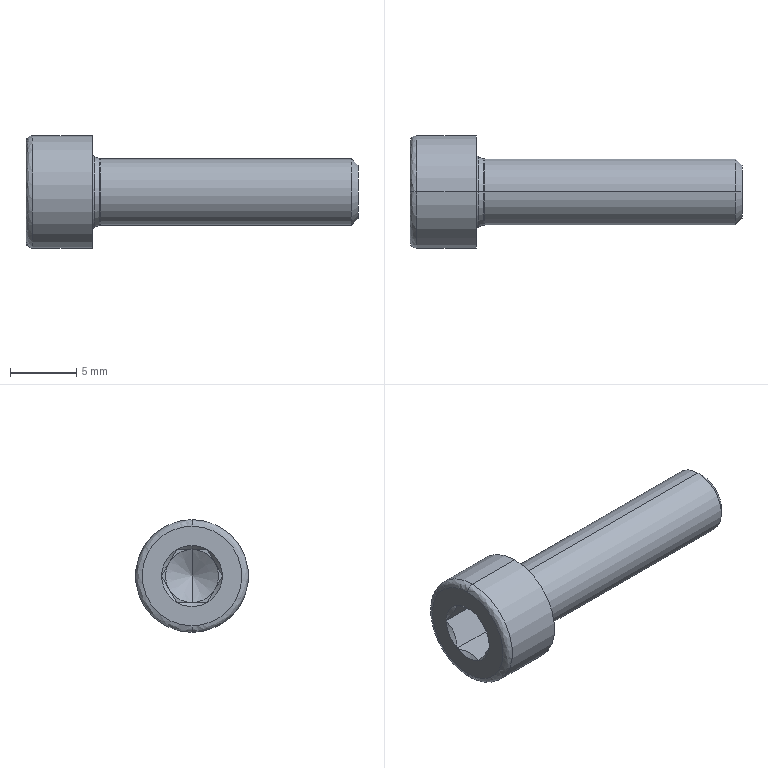Part | STEP file | _Hexagon socket head cap screw DIN 912 - M5x20 | 1 solid | 38 faces | box 25 x 8.5 x 8.5 mm | volume 626.207 mm3 | plane 15 | cone 13 | spline 6 | cylinder 4 | commonest cylinder face diameters 5 x2 8.5 x2
STEP:
#1=CARTESIAN_POINT('',(0.5298,0.,2.513));
#2=VERTEX_POINT('',#1);
#3=CARTESIAN_POINT('',(0.5298,0.,-2.513));
#4=VERTEX_POINT('',#3);
#5=CARTESIAN_POINT('',(0.5298,0.,0.));
#6=DIRECTION('',(-1.,0.,0.));
#7=DIRECTION('',(0.,0.,-1.));
#8=AXIS2_PLACEMENT_3D('',#5,#6,#7);
#9=CIRCLE('',#8,2.513);
#10=EDGE_CURVE('',#2,#4,#9,.T.);
#11=ORIENTED_EDGE('',*,*,#10,.F.);
#12=CARTESIAN_POINT('',(0.6,0.,2.5));
#13=VERTEX_POINT('',#12);
#14=CARTESIAN_POINT('',(0.6,0.,2.7));
#15=DIRECTION('',(0.,-1.,0.));
#16=DIRECTION('',(0.,0.,1.));
#17=AXIS2_PLACEMENT_3D('',#14,#15,#16);
#18=CIRCLE('',#17,0.2);
#19=EDGE_CURVE('',#2,#13,#18,.T.);
#20=ORIENTED_EDGE('',*,*,#19,.T.);
#21=CARTESIAN_POINT('',(0.6,0.,-2.5));
#22=VERTEX_POINT('',#21);
#23=CARTESIAN_POINT('',(0.6,0.,0.));
#24=DIRECTION('',(1.,0.,0.));
#25=DIRECTION('',(0.,0.,1.));
#26=AXIS2_PLACEMENT_3D('',#23,#24,#25);
#27=CIRCLE('',#26,2.5);
#28=EDGE_CURVE('',#22,#13,#27,.T.);
#29=ORIENTED_EDGE('',*,*,#28,.F.);
#30=CARTESIAN_POINT('',(0.6,0.,-2.7));
#31=DIRECTION('',(0.,1.,0.));
#32=DIRECTION('',(0.,0.,-1.));
#33=AXIS2_PLACEMENT_3D('',#30,#31,#32);
#34=CIRCLE('',#33,0.2);
#35=EDGE_CURVE('',#4,#22,#34,.T.);
#36=ORIENTED_EDGE('',*,*,#35,.F.);
#37=EDGE_LOOP('',(#11,#20,#29,#36));
#38=FACE_OUTER_BOUND('',#37,.T.);
#39=CARTESIAN_POINT('',(0.5298,0.,-2.513));
#40=CARTESIAN_POINT('',(0.5298,5.025,-2.513));
#41=CARTESIAN_POINT('',(0.5298,5.025,2.513));
#42=CARTESIAN_POINT('',(0.5298,0.,2.513));
#43=CARTESIAN_POINT('',(0.5523,0.,-2.504));
#44=CARTESIAN_POINT('',(0.5523,5.009,-2.504));
#45=CARTESIAN_POINT('',(0.5523,5.009,2.504));
#46=CARTESIAN_POINT('',(0.5523,0.,2.504));
#47=CARTESIAN_POINT('',(0.576,0.,-2.5));
#48=CARTESIAN_POINT('',(0.576,5.,-2.5));
#49=CARTESIAN_POINT('',(0.576,5.,2.5));
#50=CARTESIAN_POINT('',(0.576,0.,2.5));
#51=CARTESIAN_POINT('',(0.6,0.,-2.5));
#52=CARTESIAN_POINT('',(0.6,5.,-2.5));
#53=CARTESIAN_POINT('',(0.6,5.,2.5));
#54=CARTESIAN_POINT('',(0.6,0.,2.5));
#55=(BOUNDED_SURFACE()B_SPLINE_SURFACE(3,3,((#39,#40,#41,#42),(#43,#44,#45,#46),(#47,#48,#49,#50),(#51,#52,#53,#54)),.UNSPECIFIED.,.F.,.F.,.F.)B_SPLINE_SURFACE_WITH_KNOTS((4,4),(4,4),(0.,1.),(0.,1.),.UNSPECIFIED.)GEOMETRIC_REPRESENTATION_ITEM()RATIONAL_B_SPLINE_SURFACE(((1.,0.3333,0.3333,1.),(0.9893,0.3298,0.3298,0.9893),(0.9893,0.3298,0.3298,0.9893),(1.,0.3333,0.3333,1.)))REPRESENTATION_ITEM('')SURFACE());
#56=ADVANCED_FACE('',(#38),#55,.F.);
#57=CARTESIAN_POINT('',(0.,0.,2.85));
#58=VERTEX_POINT('',#57);
#59=CARTESIAN_POINT('',(0.,0.,-2.85));
#60=VERTEX_POINT('',#59);
#61=CARTESIAN_POINT('',(0.,0.,2.85));
#62=CARTESIAN_POINT('',(0.,0.1814,2.85));
#63=CARTESIAN_POINT('',(0.,0.4486,2.825));
#64=CARTESIAN_POINT('',(0.,0.7517,2.752));
#65=CARTESIAN_POINT('',(0.,0.9011,2.705));
#66=CARTESIAN_POINT('',(0.,0.9647,2.682));
#67=CARTESIAN_POINT('',(0.,1.007,2.666));
#68=CARTESIAN_POINT('',(0.,1.026,2.659));
#69=CARTESIAN_POINT('',(0.,1.415,2.505));
#70=CARTESIAN_POINT('',(0.,1.737,2.294));
#71=CARTESIAN_POINT('',(0.,2.154,1.876));
#72=CARTESIAN_POINT('',(0.,2.338,1.651));
#73=CARTESIAN_POINT('',(0.,2.509,1.359));
#74=CARTESIAN_POINT('',(0.,2.583,1.207));
#75=CARTESIAN_POINT('',(0.,2.612,1.14));
#76=CARTESIAN_POINT('',(0.,2.632,1.095));
#77=CARTESIAN_POINT('',(0.,2.642,1.07));
#78=CARTESIAN_POINT('',(0.,2.783,0.7118));
#79=CARTESIAN_POINT('',(0.,2.85,0.3628));
#80=CARTESIAN_POINT('',(0.,2.85,-0.1814));
#81=CARTESIAN_POINT('',(0.,2.825,-0.4486));
#82=CARTESIAN_POINT('',(0.,2.752,-0.7517));
#83=CARTESIAN_POINT('',(0.,2.705,-0.9011));
#84=CARTESIAN_POINT('',(0.,2.682,-0.9647));
#85=CARTESIAN_POINT('',(0.,2.666,-1.007));
#86=CARTESIAN_POINT('',(0.,2.659,-1.026));
#87=CARTESIAN_POINT('',(0.,2.505,-1.415));
#88=CARTESIAN_POINT('',(0.,2.294,-1.737));
#89=CARTESIAN_POINT('',(0.,1.876,-2.154));
#90=CARTESIAN_POINT('',(0.,1.651,-2.338));
#91=CARTESIAN_POINT('',(0.,1.359,-2.509));
#92=CARTESIAN_POINT('',(0.,1.207,-2.583));
#93=CARTESIAN_POINT('',(0.,1.14,-2.612));
#94=CARTESIAN_POINT('',(0.,1.095,-2.632));
#95=CARTESIAN_POINT('',(0.,1.07,-2.642));
#96=CARTESIAN_POINT('',(0.,0.7119,-2.783));
#97=CARTESIAN_POINT('',(0.,0.3622,-2.85));
#98=CARTESIAN_POINT('',(0.,0.,-2.85));
#99=B_SPLINE_CURVE_WITH_KNOTS('',3,(#61,#62,#63,#64,#65,#66,#67,#68,#69,#70,#71,#72,#73,#74,#75,#76,#77,#78,#79,#80,#81,#82,#83,#84,#85,#86,#87,#88,#89,#90,#91,#92,#93,#94,#95,#96,#97,#98),.UNSPECIFIED.,.F.,.F.,(4,1,1,1,2,2,2,1,1,1,2,2,2,1,1,1,2,2,2,1,1,1,2,2,4),(0.5,0.5312,0.5469,0.5547,0.5586,0.5625,0.625,0.6562,0.6719,0.6797,0.6836,0.6875,0.75,0.7812,0.7969,0.8047,0.8086,0.8125,0.875,0.9062,0.9219,0.9297,0.9336,0.9375,1.),.UNSPECIFIED.);
#100=EDGE_CURVE('',#58,#60,#99,.T.);
#101=ORIENTED_EDGE('',*,*,#100,.F.);
#102=CARTESIAN_POINT('',(0.1298,0.,2.663));
#103=VERTEX_POINT('',#102);
#104=CARTESIAN_POINT('',(0.2,0.,2.85));
#105=DIRECTION('',(0.,-1.,0.));
#106=DIRECTION('',(0.,0.,1.));
#107=AXIS2_PLACEMENT_3D('',#104,#105,#106);
#108=CIRCLE('',#107,0.2);
#109=EDGE_CURVE('',#58,#103,#108,.T.);
#110=ORIENTED_EDGE('',*,*,#109,.T.);
#111=CARTESIAN_POINT('',(0.1298,0.,-2.663));
#112=VERTEX_POINT('',#111);
#113=CARTESIAN_POINT('',(0.1298,0.,0.));
#114=DIRECTION('',(1.,0.,0.));
#115=DIRECTION('',(0.,0.,1.));
#116=AXIS2_PLACEMENT_3D('',#113,#114,#115);
#117=CIRCLE('',#116,2.663);
#118=EDGE_CURVE('',#112,#103,#117,.T.);
#119=ORIENTED_EDGE('',*,*,#118,.F.);
#120=CARTESIAN_POINT('',(0.2,0.,-2.85));
#121=DIRECTION('',(0.,1.,0.));
#122=DIRECTION('',(0.,0.,-1.));
#123=AXIS2_PLACEMENT_3D('',#120,#121,#122);
#124=CIRCLE('',#123,0.2);
#125=EDGE_CURVE('',#60,#112,#124,.T.);
#126=ORIENTED_EDGE('',*,*,#125,.F.);
#127=EDGE_LOOP('',(#101,#110,#119,#126));
#128=FACE_OUTER_BOUND('',#127,.T.);
#129=CARTESIAN_POINT('',(0.,0.,-2.85));
#130=CARTESIAN_POINT('',(0.,5.7,-2.85));
#131=CARTESIAN_POINT('',(0.,5.7,2.85));
#132=CARTESIAN_POINT('',(0.,0.,2.85));
#133=CARTESIAN_POINT('',(0.,0.,-2.764));
#134=CARTESIAN_POINT('',(0.,5.528,-2.764));
#135=CARTESIAN_POINT('',(0.,5.528,2.764));
#136=CARTESIAN_POINT('',(0.,0.,2.764));
#137=CARTESIAN_POINT('',(0.04909,0.,-2.693));
#138=CARTESIAN_POINT('',(0.04909,5.386,-2.693));
#139=CARTESIAN_POINT('',(0.04909,5.386,2.693));
#140=CARTESIAN_POINT('',(0.04909,0.,2.693));
#141=CARTESIAN_POINT('',(0.1298,0.,-2.663));
#142=CARTESIAN_POINT('',(0.1298,5.325,-2.663));
#143=CARTESIAN_POINT('',(0.1298,5.325,2.663));
#144=CARTESIAN_POINT('',(0.1298,0.,2.663));
#145=(BOUNDED_SURFACE()B_SPLINE_SURFACE(3,3,((#129,#130,#131,#132),(#133,#134,#135,#136),(#137,#138,#139,#140),(#141,#142,#143,#144)),.UNSPECIFIED.,.F.,.F.,.F.)B_SPLINE_SURFACE_WITH_KNOTS((4,4),(4,4),(0.,1.),(0.,1.),.UNSPECIFIED.)GEOMETRIC_REPRESENTATION_ITEM()RATIONAL_B_SPLINE_SURFACE(((1.,0.3333,0.3333,1.),(0.8813,0.2938,0.2938,0.8813),(0.8813,0.2938,0.2938,0.8813),(1.,0.3333,0.3333,1.)))REPRESENTATION_ITEM('')SURFACE());
#146=ADVANCED_FACE('',(#128),#145,.F.);
#147=CARTESIAN_POINT('',(-4.5,0.,4.25));
#148=VERTEX_POINT('',#147);
#149=CARTESIAN_POINT('',(-4.5,0.,-4.25));
#150=VERTEX_POINT('',#149);
#151=CARTESIAN_POINT('',(-4.5,0.,0.));
#152=DIRECTION('',(1.,0.,0.));
#153=DIRECTION('',(0.,0.,1.));
#154=AXIS2_PLACEMENT_3D('',#151,#152,#153);
#155=CIRCLE('',#154,4.25);
#156=EDGE_CURVE('',#148,#150,#155,.T.);
#157=ORIENTED_EDGE('',*,*,#156,.F.);
#158=CARTESIAN_POINT('',(-5.,0.,3.75));
#159=VERTEX_POINT('',#158);
#160=CARTESIAN_POINT('',(-4.5,0.,3.75));
#161=DIRECTION('',(0.,-1.,0.));
#162=DIRECTION('',(0.,0.,1.));
#163=AXIS2_PLACEMENT_3D('',#160,#161,#162);
#164=CIRCLE('',#163,0.5);
#165=EDGE_CURVE('',#148,#159,#164,.T.);
#166=ORIENTED_EDGE('',*,*,#165,.T.);
#167=CARTESIAN_POINT('',(-5.,0.,-3.75));
#168=VERTEX_POINT('',#167);
#169=CARTESIAN_POINT('',(-5.,0.,3.75));
#170=CARTESIAN_POINT('',(-5.,-7.5,3.75));
#171=CARTESIAN_POINT('',(-5.,-7.5,-3.75));
#172=CARTESIAN_POINT('',(-5.,0.,-3.75));
#173=(BOUNDED_CURVE()B_SPLINE_CURVE(3,(#169,#170,#171,#172),.UNSPECIFIED.,.F.,.T.)B_SPLINE_CURVE_WITH_KNOTS((4,4),(0.5,1.),.UNSPECIFIED.)CURVE()GEOMETRIC_REPRESENTATION_ITEM()RATIONAL_B_SPLINE_CURVE((1.,0.3333,0.3333,1.))REPRESENTATION_ITEM(''));
#174=EDGE_CURVE('',#159,#168,#173,.T.);
#175=ORIENTED_EDGE('',*,*,#174,.T.);
#176=CARTESIAN_POINT('',(-4.5,0.,-3.75));
#177=DIRECTION('',(0.,1.,0.));
#178=DIRECTION('',(0.,0.,-1.));
#179=AXIS2_PLACEMENT_3D('',#176,#177,#178);
#180=CIRCLE('',#179,0.5);
#181=EDGE_CURVE('',#150,#168,#180,.T.);
#182=ORIENTED_EDGE('',*,*,#181,.F.);
#183=EDGE_LOOP('',(#157,#166,#175,#182));
#184=FACE_OUTER_BOUND('',#183,.T.);
#185=CARTESIAN_POINT('',(-4.5,0.,4.25));
#186=CARTESIAN_POINT('',(-4.5,-8.5,4.25));
#187=CARTESIAN_POINT('',(-4.5,-8.5,-4.25));
#188=CARTESIAN_POINT('',(-4.5,0.,-4.25));
#189=CARTESIAN_POINT('',(-4.793,0.,4.25));
#190=CARTESIAN_POINT('',(-4.793,-8.5,4.25));
#191=CARTESIAN_POINT('',(-4.793,-8.5,-4.25));
#192=CARTESIAN_POINT('',(-4.793,0.,-4.25));
#193=CARTESIAN_POINT('',(-5.,0.,4.043));
#194=CARTESIAN_POINT('',(-5.,-8.086,4.043));
#195=CARTESIAN_POINT('',(-5.,-8.086,-4.043));
#196=CARTESIAN_POINT('',(-5.,0.,-4.043));
#197=CARTESIAN_POINT('',(-5.,0.,3.75));
#198=CARTESIAN_POINT('',(-5.,-7.5,3.75));
#199=CARTESIAN_POINT('',(-5.,-7.5,-3.75));
#200=CARTESIAN_POINT('',(-5.,0.,-3.75));
#201=(BOUNDED_SURFACE()B_SPLINE_SURFACE(3,3,((#185,#186,#187,#188),(#189,#190,#191,#192),(#193,#194,#195,#196),(#197,#198,#199,#200)),.UNSPECIFIED.,.F.,.F.,.F.)B_SPLINE_SURFACE_WITH_KNOTS((4,4),(4,4),(0.,1.),(0.,1.),.UNSPECIFIED.)GEOMETRIC_REPRESENTATION_ITEM()RATIONAL_B_SPLINE_SURFACE(((1.,0.3333,0.3333,1.),(0.8047,0.2682,0.2682,0.8047),(0.8047,0.2682,0.2682,0.8047),(1.,0.3333,0.3333,1.)))REPRESENTATION_ITEM('')SURFACE());
#202=ADVANCED_FACE('',(#184),#201,.T.);
#203=CARTESIAN_POINT('',(19.509,0.,2.5));
#204=VERTEX_POINT('',#203);
#205=CARTESIAN_POINT('',(19.509,0.,-2.5));
#206=VERTEX_POINT('',#205);
#207=CARTESIAN_POINT('',(19.509,0.,0.));
#208=DIRECTION('',(-1.,0.,0.));
#209=DIRECTION('',(0.,0.,1.));
#210=AXIS2_PLACEMENT_3D('',#207,#208,#209);
#211=CIRCLE('',#210,2.5);
#212=EDGE_CURVE('',#204,#206,#211,.T.);
#213=ORIENTED_EDGE('',*,*,#212,.T.);
#214=CARTESIAN_POINT('',(23.,0.,-2.5));
#215=DIRECTION('',(-1.,0.,0.));
#216=VECTOR('',#215,1000.);
#217=LINE('',#214,#216);
#218=EDGE_CURVE('',#206,#22,#217,.T.);
#219=ORIENTED_EDGE('',*,*,#218,.T.);
#220=ORIENTED_EDGE('',*,*,#28,.T.);
#221=CARTESIAN_POINT('',(23.,0.,2.5));
#222=DIRECTION('',(-1.,0.,0.));
#223=VECTOR('',#222,1000.);
#224=LINE('',#221,#223);
#225=EDGE_CURVE('',#204,#13,#224,.T.);
#226=ORIENTED_EDGE('',*,*,#225,.F.);
#227=EDGE_LOOP('',(#213,#219,#220,#226));
#228=FACE_OUTER_BOUND('',#227,.T.);
#229=CARTESIAN_POINT('',(23.,0.,0.));
#230=DIRECTION('',(-1.,0.,0.));
#231=DIRECTION('',(0.,0.,1.));
#232=AXIS2_PLACEMENT_3D('',#229,#230,#231);
#233=CYLINDRICAL_SURFACE('',#232,2.5);
#234=ADVANCED_FACE('',(#228),#233,.T.);
#235=CARTESIAN_POINT('',(20.,0.,2.009));
#236=VERTEX_POINT('',#235);
#237=CARTESIAN_POINT('',(20.,0.,-2.009));
#238=VERTEX_POINT('',#237);
#239=CARTESIAN_POINT('',(20.,0.,0.));
#240=DIRECTION('',(-1.,0.,0.));
#241=DIRECTION('',(0.,0.,1.));
#242=AXIS2_PLACEMENT_3D('',#239,#240,#241);
#243=CIRCLE('',#242,2.009);
#244=EDGE_CURVE('',#236,#238,#243,.T.);
#245=ORIENTED_EDGE('',*,*,#244,.T.);
#246=CARTESIAN_POINT('',(19.509,0.,-2.5));
#247=DIRECTION('',(-0.7071,0.,-0.7071));
#248=VECTOR('',#247,1000.);
#249=LINE('',#246,#248);
#250=EDGE_CURVE('',#238,#206,#249,.T.);
#251=ORIENTED_EDGE('',*,*,#250,.T.);
#252=ORIENTED_EDGE('',*,*,#212,.F.);
#253=CARTESIAN_POINT('',(19.509,0.,2.5));
#254=DIRECTION('',(-0.7071,0.,0.7071));
#255=VECTOR('',#254,1000.);
#256=LINE('',#253,#255);
#257=EDGE_CURVE('',#236,#204,#256,.T.);
#258=ORIENTED_EDGE('',*,*,#257,.F.);
#259=EDGE_LOOP('',(#245,#251,#252,#258));
#260=FACE_OUTER_BOUND('',#259,.T.);
#261=CARTESIAN_POINT('',(19.509,0.,0.));
#262=DIRECTION('',(-1.,0.,0.));
#263=DIRECTION('',(0.,0.,1.));
#264=AXIS2_PLACEMENT_3D('',#261,#262,#263);
#265=CONICAL_SURFACE('',#264,2.5,0.7854);
#266=ADVANCED_FACE('',(#260),#265,.T.);
#267=ORIENTED_EDGE('',*,*,#10,.T.);
#268=CARTESIAN_POINT('',(0.1298,0.,-2.663));
#269=DIRECTION('',(-0.9363,0.,-0.3511));
#270=VECTOR('',#269,1000.);
#271=LINE('',#268,#270);
#272=EDGE_CURVE('',#4,#112,#271,.T.);
#273=ORIENTED_EDGE('',*,*,#272,.T.);
#274=ORIENTED_EDGE('',*,*,#118,.T.);
#275=CARTESIAN_POINT('',(0.1298,0.,2.663));
#276=DIRECTION('',(-0.9363,0.,0.3511));
#277=VECTOR('',#276,1000.);
#278=LINE('',#275,#277);
#279=EDGE_CURVE('',#2,#103,#278,.T.);
#280=ORIENTED_EDGE('',*,*,#279,.F.);
#281=EDGE_LOOP('',(#267,#273,#274,#280));
#282=FACE_OUTER_BOUND('',#281,.T.);
#283=CARTESIAN_POINT('',(0.1298,0.,0.));
#284=DIRECTION('',(-1.,0.,0.));
#285=DIRECTION('',(0.,0.,1.));
#286=AXIS2_PLACEMENT_3D('',#283,#284,#285);
#287=CONICAL_SURFACE('',#286,2.663,0.3588);
#288=ADVANCED_FACE('',(#282),#287,.T.);
#289=CARTESIAN_POINT('',(0.,0.,4.25));
#290=VERTEX_POINT('',#289);
#291=CARTESIAN_POINT('',(0.,0.,-4.25));
#292=VERTEX_POINT('',#291);
#293=CARTESIAN_POINT('',(0.,0.,0.));
#294=DIRECTION('',(-1.,0.,0.));
#295=DIRECTION('',(0.,0.,1.));
#296=AXIS2_PLACEMENT_3D('',#293,#294,#295);
#297=CIRCLE('',#296,4.25);
#298=EDGE_CURVE('',#290,#292,#297,.T.);
#299=ORIENTED_EDGE('',*,*,#298,.T.);
#300=CARTESIAN_POINT('',(23.,0.,-4.25));
#301=DIRECTION('',(-1.,0.,0.));
#302=VECTOR('',#301,1000.);
#303=LINE('',#300,#302);
#304=EDGE_CURVE('',#292,#150,#303,.T.);
#305=ORIENTED_EDGE('',*,*,#304,.T.);
#306=CARTESIAN_POINT('',(-4.5,0.,0.));
#307=DIRECTION('',(1.,0.,0.));
#308=DIRECTION('',(0.,0.,1.));
#309=AXIS2_PLACEMENT_3D('',#306,#307,#308);
#310=CIRCLE('',#309,4.25);
#311=EDGE_CURVE('',#150,#148,#310,.T.);
#312=ORIENTED_EDGE('',*,*,#311,.T.);
#313=CARTESIAN_POINT('',(23.,0.,4.25));
#314=DIRECTION('',(-1.,0.,0.));
#315=VECTOR('',#314,1000.);
#316=LINE('',#313,#315);
#317=EDGE_CURVE('',#290,#148,#316,.T.);
#318=ORIENTED_EDGE('',*,*,#317,.F.);
#319=EDGE_LOOP('',(#299,#305,#312,#318));
#320=FACE_OUTER_BOUND('',#319,.T.);
#321=CARTESIAN_POINT('',(23.,0.,0.));
#322=DIRECTION('',(-1.,0.,0.));
#323=DIRECTION('',(0.,0.,1.));
#324=AXIS2_PLACEMENT_3D('',#321,#322,#323);
#325=CYLINDRICAL_SURFACE('',#324,4.25);
#326=ADVANCED_FACE('',(#320),#325,.T.);
#327=CARTESIAN_POINT('',(-4.71,0.,2.));
#328=VERTEX_POINT('',#327);
#329=CARTESIAN_POINT('',(-5.,1.115,2.));
#330=VERTEX_POINT('',#329);
#331=CARTESIAN_POINT('',(-4.71,0.,2.));
#332=CARTESIAN_POINT('',(-4.71,0.3872,2.));
#333=CARTESIAN_POINT('',(-4.829,0.765,2.));
#334=CARTESIAN_POINT('',(-5.,1.115,2.));
#335=B_SPLINE_CURVE_WITH_KNOTS('',3,(#331,#332,#333,#334),.UNSPECIFIED.,.F.,.F.,(4,4),(0.001154,0.0023),.UNSPECIFIED.);
#336=EDGE_CURVE('',#328,#330,#335,.T.);
#337=ORIENTED_EDGE('',*,*,#336,.F.);
#338=CARTESIAN_POINT('',(-5.,0.,2.29));
#339=VERTEX_POINT('',#338);
#340=CARTESIAN_POINT('',(-5.,0.,2.29));
#341=DIRECTION('',(-0.7071,0.,0.7071));
#342=VECTOR('',#341,1000.);
#343=LINE('',#340,#342);
#344=EDGE_CURVE('',#328,#339,#343,.T.);
#345=ORIENTED_EDGE('',*,*,#344,.T.);
#346=CARTESIAN_POINT('',(-5.,0.,0.));
#347=DIRECTION('',(-1.,0.,0.));
#348=DIRECTION('',(0.,0.,1.));
#349=AXIS2_PLACEMENT_3D('',#346,#347,#348);
#350=CIRCLE('',#349,2.29);
#351=EDGE_CURVE('',#339,#330,#350,.T.);
#352=ORIENTED_EDGE('',*,*,#351,.T.);
#353=EDGE_LOOP('',(#337,#345,#352));
#354=FACE_OUTER_BOUND('',#353,.T.);
#355=CARTESIAN_POINT('',(-5.,0.,0.));
#356=DIRECTION('',(-1.,0.,0.));
#357=DIRECTION('',(0.,0.,1.));
#358=AXIS2_PLACEMENT_3D('',#355,#356,#357);
#359=CONICAL_SURFACE('',#358,2.29,0.7854);
#360=ADVANCED_FACE('',(#354),#359,.F.);
#361=CARTESIAN_POINT('',(-0.7453,0.,0.));
#362=VERTEX_POINT('',#361);
#363=CARTESIAN_POINT('',(-1.9,0.,2.));
#364=VERTEX_POINT('',#363);
#365=CARTESIAN_POINT('',(-1.9,0.,2.));
#366=DIRECTION('',(-0.5,0.,0.866));
#367=VECTOR('',#366,1000.);
#368=LINE('',#365,#367);
#369=EDGE_CURVE('',#362,#364,#368,.T.);
#370=ORIENTED_EDGE('',*,*,#369,.F.);
#371=CARTESIAN_POINT('',(-1.9,0.,-2.));
#372=VERTEX_POINT('',#371);
#373=CARTESIAN_POINT('',(-1.9,0.,-2.));
#374=DIRECTION('',(-0.5,0.,-0.866));
#375=VECTOR('',#374,1000.);
#376=LINE('',#373,#375);
#377=EDGE_CURVE('',#362,#372,#376,.T.);
#378=ORIENTED_EDGE('',*,*,#377,.T.);
#379=CARTESIAN_POINT('',(-1.9,-1.732,-1.));
#380=VERTEX_POINT('',#379);
#381=CARTESIAN_POINT('',(-1.9,0.,0.));
#382=DIRECTION('',(1.,0.,0.));
#383=DIRECTION('',(0.,0.,1.));
#384=AXIS2_PLACEMENT_3D('',#381,#382,#383);
#385=CIRCLE('',#384,2.);
#386=EDGE_CURVE('',#380,#372,#385,.T.);
#387=ORIENTED_EDGE('',*,*,#386,.F.);
#388=CARTESIAN_POINT('',(-1.9,-1.732,1.));
#389=VERTEX_POINT('',#388);
#390=CARTESIAN_POINT('',(-1.9,0.,0.));
#391=DIRECTION('',(1.,0.,0.));
#392=DIRECTION('',(0.,0.,1.));
#393=AXIS2_PLACEMENT_3D('',#390,#391,#392);
#394=CIRCLE('',#393,2.);
#395=EDGE_CURVE('',#389,#380,#394,.T.);
#396=ORIENTED_EDGE('',*,*,#395,.F.);
#397=CARTESIAN_POINT('',(-1.9,0.,0.));
#398=DIRECTION('',(1.,0.,0.));
#399=DIRECTION('',(0.,0.,1.));
#400=AXIS2_PLACEMENT_3D('',#397,#398,#399);
#401=CIRCLE('',#400,2.);
#402=EDGE_CURVE('',#364,#389,#401,.T.);
#403=ORIENTED_EDGE('',*,*,#402,.F.);
#404=EDGE_LOOP('',(#370,#378,#387,#396,#403));
#405=FACE_OUTER_BOUND('',#404,.T.);
#406=CARTESIAN_POINT('',(-1.9,0.,0.));
#407=DIRECTION('',(-1.,0.,0.));
#408=DIRECTION('',(0.,0.,1.));
#409=AXIS2_PLACEMENT_3D('',#406,#407,#408);
#410=CONICAL_SURFACE('',#409,2.,1.047);
#411=ADVANCED_FACE('',(#405),#410,.F.);
#412=ORIENTED_EDGE('',*,*,#218,.F.);
#413=CARTESIAN_POINT('',(19.509,0.,0.));
#414=DIRECTION('',(-1.,0.,0.));
#415=DIRECTION('',(0.,0.,1.));
#416=AXIS2_PLACEMENT_3D('',#413,#414,#415);
#417=CIRCLE('',#416,2.5);
#418=EDGE_CURVE('',#206,#204,#417,.T.);
#419=ORIENTED_EDGE('',*,*,#418,.T.);
#420=ORIENTED_EDGE('',*,*,#225,.T.);
#421=CARTESIAN_POINT('',(0.6,0.,0.));
#422=DIRECTION('',(1.,0.,0.));
#423=DIRECTION('',(0.,0.,1.));
#424=AXIS2_PLACEMENT_3D('',#421,#422,#423);
#425=CIRCLE('',#424,2.5);
#426=EDGE_CURVE('',#13,#22,#425,.T.);
#427=ORIENTED_EDGE('',*,*,#426,.T.);
#428=EDGE_LOOP('',(#412,#419,#420,#427));
#429=FACE_OUTER_BOUND('',#428,.T.);
#430=CARTESIAN_POINT('',(23.,0.,0.));
#431=DIRECTION('',(-1.,0.,0.));
#432=DIRECTION('',(0.,0.,1.));
#433=AXIS2_PLACEMENT_3D('',#430,#431,#432);
#434=CYLINDRICAL_SURFACE('',#433,2.5);
#435=ADVANCED_FACE('',(#429),#434,.T.);
#436=ORIENTED_EDGE('',*,*,#19,.F.);
#437=CARTESIAN_POINT('',(0.5298,0.,0.));
#438=DIRECTION('',(-1.,0.,0.));
#439=DIRECTION('',(0.,0.,-1.));
#440=AXIS2_PLACEMENT_3D('',#437,#438,#439);
#441=CIRCLE('',#440,2.513);
#442=EDGE_CURVE('',#4,#2,#441,.T.);
#443=ORIENTED_EDGE('',*,*,#442,.F.);
#444=ORIENTED_EDGE('',*,*,#35,.T.);
#445=ORIENTED_EDGE('',*,*,#426,.F.);
#446=EDGE_LOOP('',(#436,#443,#444,#445));
#447=FACE_OUTER_BOUND('',#446,.T.);
#448=CARTESIAN_POINT('',(0.5298,0.,2.513));
#449=CARTESIAN_POINT('',(0.5298,-5.025,2.513));
#450=CARTESIAN_POINT('',(0.5298,-5.025,-2.513));
#451=CARTESIAN_POINT('',(0.5298,0.,-2.513));
#452=CARTESIAN_POINT('',(0.5523,0.,2.504));
#453=CARTESIAN_POINT('',(0.5523,-5.009,2.504));
#454=CARTESIAN_POINT('',(0.5523,-5.009,-2.504));
#455=CARTESIAN_POINT('',(0.5523,0.,-2.504));
#456=CARTESIAN_POINT('',(0.576,0.,2.5));
#457=CARTESIAN_POINT('',(0.576,-5.,2.5));
#458=CARTESIAN_POINT('',(0.576,-5.,-2.5));
#459=CARTESIAN_POINT('',(0.576,0.,-2.5));
#460=CARTESIAN_POINT('',(0.6,0.,2.5));
#461=CARTESIAN_POINT('',(0.6,-5.,2.5));
#462=CARTESIAN_POINT('',(0.6,-5.,-2.5));
#463=CARTESIAN_POINT('',(0.6,0.,-2.5));
#464=(BOUNDED_SURFACE()B_SPLINE_SURFACE(3,3,((#448,#449,#450,#451),(#452,#453,#454,#455),(#456,#457,#458,#459),(#460,#461,#462,#463)),.UNSPECIFIED.,.F.,.F.,.F.)B_SPLINE_SURFACE_WITH_KNOTS((4,4),(4,4),(0.,1.),(0.,1.),.UNSPECIFIED.)GEOMETRIC_REPRESENTATION_ITEM()RATIONAL_B_SPLINE_SURFACE(((1.,0.3333,0.3333,1.),(0.9893,0.3298,0.3298,0.9893),(0.9893,0.3298,0.3298,0.9893),(1.,0.3333,0.3333,1.)))REPRESENTATION_ITEM('')SURFACE());
#465=ADVANCED_FACE('',(#447),#464,.F.);
#466=ORIENTED_EDGE('',*,*,#250,.F.);
#467=CARTESIAN_POINT('',(20.,0.,0.));
#468=DIRECTION('',(-1.,0.,0.));
#469=DIRECTION('',(0.,0.,1.));
#470=AXIS2_PLACEMENT_3D('',#467,#468,#469);
#471=CIRCLE('',#470,2.009);
#472=EDGE_CURVE('',#238,#236,#471,.T.);
#473=ORIENTED_EDGE('',*,*,#472,.T.);
#474=ORIENTED_EDGE('',*,*,#257,.T.);
#475=ORIENTED_EDGE('',*,*,#418,.F.);
#476=EDGE_LOOP('',(#466,#473,#474,#475));
#477=FACE_OUTER_BOUND('',#476,.T.);
#478=CARTESIAN_POINT('',(19.509,0.,0.));
#479=DIRECTION('',(-1.,0.,0.));
#480=DIRECTION('',(0.,0.,1.));
#481=AXIS2_PLACEMENT_3D('',#478,#479,#480);
#482=CONICAL_SURFACE('',#481,2.5,0.7854);
#483=ADVANCED_FACE('',(#477),#482,.T.);
#484=ORIENTED_EDGE('',*,*,#272,.F.);
#485=ORIENTED_EDGE('',*,*,#442,.T.);
#486=ORIENTED_EDGE('',*,*,#279,.T.);
#487=CARTESIAN_POINT('',(0.1298,0.,0.));
#488=DIRECTION('',(1.,0.,0.));
#489=DIRECTION('',(0.,0.,1.));
#490=AXIS2_PLACEMENT_3D('',#487,#488,#489);
#491=CIRCLE('',#490,2.663);
#492=EDGE_CURVE('',#103,#112,#491,.T.);
#493=ORIENTED_EDGE('',*,*,#492,.T.);
#494=EDGE_LOOP('',(#484,#485,#486,#493));
#495=FACE_OUTER_BOUND('',#494,.T.);
#496=CARTESIAN_POINT('',(0.1298,0.,0.));
#497=DIRECTION('',(-1.,0.,0.));
#498=DIRECTION('',(0.,0.,1.));
#499=AXIS2_PLACEMENT_3D('',#496,#497,#498);
#500=CONICAL_SURFACE('',#499,2.663,0.3588);
#501=ADVANCED_FACE('',(#495),#500,.T.);
#502=ORIENTED_EDGE('',*,*,#244,.F.);
#503=ORIENTED_EDGE('',*,*,#472,.F.);
#504=EDGE_LOOP('',(#502,#503));
#505=FACE_OUTER_BOUND('',#504,.T.);
#506=CARTESIAN_POINT('',(20.,2.01,0.));
#507=DIRECTION('',(-1.,0.,0.));
#508=DIRECTION('',(0.,0.,1.));
#509=AXIS2_PLACEMENT_3D('',#506,#507,#508);
#510=PLANE('',#509);
#511=ADVANCED_FACE('',(#505),#510,.F.);
#512=ORIENTED_EDGE('',*,*,#109,.F.);
#513=CARTESIAN_POINT('',(0.,0.,-2.85));
#514=CARTESIAN_POINT('',(0.,-0.1813,-2.85));
#515=CARTESIAN_POINT('',(0.,-0.4484,-2.825));
#516=CARTESIAN_POINT('',(0.,-0.7516,-2.752));
#517=CARTESIAN_POINT('',(0.,-0.901,-2.705));
#518=CARTESIAN_POINT('',(0.,-0.9646,-2.682));
#519=CARTESIAN_POINT('',(0.,-1.007,-2.666));
#520=CARTESIAN_POINT('',(0.,-1.026,-2.659));
#521=CARTESIAN_POINT('',(0.,-1.415,-2.505));
#522=CARTESIAN_POINT('',(0.,-1.737,-2.294));
#523=CARTESIAN_POINT('',(0.,-2.154,-1.876));
#524=CARTESIAN_POINT('',(0.,-2.338,-1.651));
#525=CARTESIAN_POINT('',(0.,-2.509,-1.359));
#526=CARTESIAN_POINT('',(0.,-2.583,-1.207));
#527=CARTESIAN_POINT('',(0.,-2.612,-1.14));
#528=CARTESIAN_POINT('',(0.,-2.632,-1.095));
#529=CARTESIAN_POINT('',(0.,-2.642,-1.07));
#530=CARTESIAN_POINT('',(0.,-2.783,-0.7118));
#531=CARTESIAN_POINT('',(0.,-2.85,-0.3628));
#532=CARTESIAN_POINT('',(0.,-2.85,0.1814));
#533=CARTESIAN_POINT('',(0.,-2.825,0.4486));
#534=CARTESIAN_POINT('',(0.,-2.752,0.7517));
#535=CARTESIAN_POINT('',(0.,-2.705,0.9011));
#536=CARTESIAN_POINT('',(0.,-2.682,0.9647));
#537=CARTESIAN_POINT('',(0.,-2.666,1.007));
#538=CARTESIAN_POINT('',(0.,-2.659,1.026));
#539=CARTESIAN_POINT('',(0.,-2.505,1.415));
#540=CARTESIAN_POINT('',(0.,-2.294,1.737));
#541=CARTESIAN_POINT('',(0.,-1.876,2.154));
#542=CARTESIAN_POINT('',(0.,-1.651,2.338));
#543=CARTESIAN_POINT('',(0.,-1.359,2.509));
#544=CARTESIAN_POINT('',(0.,-1.207,2.583));
#545=CARTESIAN_POINT('',(0.,-1.14,2.612));
#546=CARTESIAN_POINT('',(0.,-1.095,2.632));
#547=CARTESIAN_POINT('',(0.,-1.07,2.642));
#548=CARTESIAN_POINT('',(0.,-0.7118,2.783));
#549=CARTESIAN_POINT('',(0.,-0.3628,2.85));
#550=CARTESIAN_POINT('',(0.,0.,2.85));
#551=B_SPLINE_CURVE_WITH_KNOTS('',3,(#513,#514,#515,#516,#517,#518,#519,#520,#521,#522,#523,#524,#525,#526,#527,#528,#529,#530,#531,#532,#533,#534,#535,#536,#537,#538,#539,#540,#541,#542,#543,#544,#545,#546,#547,#548,#549,#550),.UNSPECIFIED.,.F.,.F.,(4,1,1,1,2,2,2,1,1,1,2,2,2,1,1,1,2,2,2,1,1,1,2,2,4),(0.,0.03125,0.04687,0.05469,0.05859,0.0625,0.125,0.1563,0.1719,0.1797,0.1836,0.1875,0.25,0.2813,0.2969,0.3047,0.3086,0.3125,0.375,0.4063,0.4219,0.4297,0.4336,0.4375,0.5),.UNSPECIFIED.);
#552=EDGE_CURVE('',#60,#58,#551,.T.);
#553=ORIENTED_EDGE('',*,*,#552,.F.);
#554=ORIENTED_EDGE('',*,*,#125,.T.);
#555=ORIENTED_EDGE('',*,*,#492,.F.);
#556=EDGE_LOOP('',(#512,#553,#554,#555));
#557=FACE_OUTER_BOUND('',#556,.T.);
#558=CARTESIAN_POINT('',(0.,0.,2.85));
#559=CARTESIAN_POINT('',(0.,-5.7,2.85));
#560=CARTESIAN_POINT('',(0.,-5.7,-2.85));
#561=CARTESIAN_POINT('',(0.,0.,-2.85));
#562=CARTESIAN_POINT('',(0.,0.,2.764));
#563=CARTESIAN_POINT('',(0.,-5.528,2.764));
#564=CARTESIAN_POINT('',(0.,-5.528,-2.764));
#565=CARTESIAN_POINT('',(0.,0.,-2.764));
#566=CARTESIAN_POINT('',(0.04909,0.,2.693));
#567=CARTESIAN_POINT('',(0.04909,-5.386,2.693));
#568=CARTESIAN_POINT('',(0.04909,-5.386,-2.693));
#569=CARTESIAN_POINT('',(0.04909,0.,-2.693));
#570=CARTESIAN_POINT('',(0.1298,0.,2.663));
#571=CARTESIAN_POINT('',(0.1298,-5.325,2.663));
#572=CARTESIAN_POINT('',(0.1298,-5.325,-2.663));
#573=CARTESIAN_POINT('',(0.1298,0.,-2.663));
#574=(BOUNDED_SURFACE()B_SPLINE_SURFACE(3,3,((#558,#559,#560,#561),(#562,#563,#564,#565),(#566,#567,#568,#569),(#570,#571,#572,#573)),.UNSPECIFIED.,.F.,.F.,.F.)B_SPLINE_SURFACE_WITH_KNOTS((4,4),(4,4),(0.,1.),(0.,1.),.UNSPECIFIED.)GEOMETRIC_REPRESENTATION_ITEM()RATIONAL_B_SPLINE_SURFACE(((1.,0.3333,0.3333,1.),(0.8813,0.2938,0.2938,0.8813),(0.8813,0.2938,0.2938,0.8813),(1.,0.3333,0.3333,1.)))REPRESENTATION_ITEM('')SURFACE());
#575=ADVANCED_FACE('',(#557),#574,.F.);
#576=ORIENTED_EDGE('',*,*,#298,.F.);
#577=CARTESIAN_POINT('',(0.,0.,0.));
#578=DIRECTION('',(-1.,0.,0.));
#579=DIRECTION('',(0.,0.,1.));
#580=AXIS2_PLACEMENT_3D('',#577,#578,#579);
#581=CIRCLE('',#580,4.25);
#582=EDGE_CURVE('',#292,#290,#581,.T.);
#583=ORIENTED_EDGE('',*,*,#582,.F.);
#584=EDGE_LOOP('',(#576,#583));
#585=FACE_OUTER_BOUND('',#584,.T.);
#586=ORIENTED_EDGE('',*,*,#552,.T.);
#587=ORIENTED_EDGE('',*,*,#100,.T.);
#588=EDGE_LOOP('',(#586,#587));
#589=FACE_BOUND('',#588,.T.);
#590=CARTESIAN_POINT('',(0.,4.25,0.));
#591=DIRECTION('',(-1.,0.,0.));
#592=DIRECTION('',(0.,0.,1.));
#593=AXIS2_PLACEMENT_3D('',#590,#591,#592);
#594=PLANE('',#593);
#595=ADVANCED_FACE('',(#585,#589),#594,.F.);
#596=ORIENTED_EDGE('',*,*,#304,.F.);
#597=ORIENTED_EDGE('',*,*,#582,.T.);
#598=ORIENTED_EDGE('',*,*,#317,.T.);
#599=ORIENTED_EDGE('',*,*,#156,.T.);
#600=EDGE_LOOP('',(#596,#597,#598,#599));
#601=FACE_OUTER_BOUND('',#600,.T.);
#602=CARTESIAN_POINT('',(23.,0.,0.));
#603=DIRECTION('',(-1.,0.,0.));
#604=DIRECTION('',(0.,0.,1.));
#605=AXIS2_PLACEMENT_3D('',#602,#603,#604);
#606=CYLINDRICAL_SURFACE('',#605,4.25);
#607=ADVANCED_FACE('',(#601),#606,.T.);
#608=ORIENTED_EDGE('',*,*,#165,.F.);
#609=ORIENTED_EDGE('',*,*,#311,.F.);
#610=ORIENTED_EDGE('',*,*,#181,.T.);
#611=CARTESIAN_POINT('',(-5.,0.,-3.75));
#612=CARTESIAN_POINT('',(-5.,7.5,-3.75));
#613=CARTESIAN_POINT('',(-5.,7.5,3.75));
#614=CARTESIAN_POINT('',(-5.,0.,3.75));
#615=(BOUNDED_CURVE()B_SPLINE_CURVE(3,(#611,#612,#613,#614),.UNSPECIFIED.,.F.,.F.)B_SPLINE_CURVE_WITH_KNOTS((4,4),(0.,0.5),.UNSPECIFIED.)CURVE()GEOMETRIC_REPRESENTATION_ITEM()RATIONAL_B_SPLINE_CURVE((1.,0.3333,0.3333,1.))REPRESENTATION_ITEM(''));
#616=EDGE_CURVE('',#168,#159,#615,.T.);
#617=ORIENTED_EDGE('',*,*,#616,.T.);
#618=EDGE_LOOP('',(#608,#609,#610,#617));
#619=FACE_OUTER_BOUND('',#618,.T.);
#620=CARTESIAN_POINT('',(-4.5,0.,-4.25));
#621=CARTESIAN_POINT('',(-4.5,8.5,-4.25));
#622=CARTESIAN_POINT('',(-4.5,8.5,4.25));
#623=CARTESIAN_POINT('',(-4.5,0.,4.25));
#624=CARTESIAN_POINT('',(-4.793,0.,-4.25));
#625=CARTESIAN_POINT('',(-4.793,8.5,-4.25));
#626=CARTESIAN_POINT('',(-4.793,8.5,4.25));
#627=CARTESIAN_POINT('',(-4.793,0.,4.25));
#628=CARTESIAN_POINT('',(-5.,0.,-4.043));
#629=CARTESIAN_POINT('',(-5.,8.086,-4.043));
#630=CARTESIAN_POINT('',(-5.,8.086,4.043));
#631=CARTESIAN_POINT('',(-5.,0.,4.043));
#632=CARTESIAN_POINT('',(-5.,0.,-3.75));
#633=CARTESIAN_POINT('',(-5.,7.5,-3.75));
#634=CARTESIAN_POINT('',(-5.,7.5,3.75));
#635=CARTESIAN_POINT('',(-5.,0.,3.75));
#636=(BOUNDED_SURFACE()B_SPLINE_SURFACE(3,3,((#620,#621,#622,#623),(#624,#625,#626,#627),(#628,#629,#630,#631),(#632,#633,#634,#635)),.UNSPECIFIED.,.F.,.F.,.F.)B_SPLINE_SURFACE_WITH_KNOTS((4,4),(4,4),(0.,1.),(0.,1.),.UNSPECIFIED.)GEOMETRIC_REPRESENTATION_ITEM()RATIONAL_B_SPLINE_SURFACE(((1.,0.3333,0.3333,1.),(0.8047,0.2682,0.2682,0.8047),(0.8047,0.2682,0.2682,0.8047),(1.,0.3333,0.3333,1.)))REPRESENTATION_ITEM('')SURFACE());
#637=ADVANCED_FACE('',(#619),#636,.T.);
#638=CARTESIAN_POINT('',(-5.,-1.115,2.));
#639=VERTEX_POINT('',#638);
#640=CARTESIAN_POINT('',(-5.,-1.155,2.));
#641=VERTEX_POINT('',#640);
#642=CARTESIAN_POINT('',(-5.,1.155,2.));
#643=DIRECTION('',(0.,-1.,0.));
#644=VECTOR('',#643,1000.);
#645=LINE('',#642,#644);
#646=EDGE_CURVE('',#639,#641,#645,.T.);
#647=ORIENTED_EDGE('',*,*,#646,.T.);
#648=CARTESIAN_POINT('',(-5.,-1.174,1.966));
#649=VERTEX_POINT('',#648);
#650=CARTESIAN_POINT('',(-5.,-1.155,2.));
#651=DIRECTION('',(0.,-0.5,-0.866));
#652=VECTOR('',#651,1000.);
#653=LINE('',#650,#652);
#654=EDGE_CURVE('',#641,#649,#653,.T.);
#655=ORIENTED_EDGE('',*,*,#654,.T.);
#656=CARTESIAN_POINT('',(-5.,-2.29,0.03404));
#657=VERTEX_POINT('',#656);
#658=CARTESIAN_POINT('',(-5.,0.,0.));
#659=DIRECTION('',(-1.,0.,0.));
#660=DIRECTION('',(0.,0.,1.));
#661=AXIS2_PLACEMENT_3D('',#658,#659,#660);
#662=CIRCLE('',#661,2.29);
#663=EDGE_CURVE('',#657,#649,#662,.T.);
#664=ORIENTED_EDGE('',*,*,#663,.F.);
#665=CARTESIAN_POINT('',(-5.,-2.309,0.));
#666=VERTEX_POINT('',#665);
#667=CARTESIAN_POINT('',(-5.,-1.155,2.));
#668=DIRECTION('',(0.,-0.5,-0.866));
#669=VECTOR('',#668,1000.);
#670=LINE('',#667,#669);
#671=EDGE_CURVE('',#657,#666,#670,.T.);
#672=ORIENTED_EDGE('',*,*,#671,.T.);
#673=CARTESIAN_POINT('',(-5.,-2.29,-0.03404));
#674=VERTEX_POINT('',#673);
#675=CARTESIAN_POINT('',(-5.,-2.309,0.));
#676=DIRECTION('',(0.,0.5,-0.866));
#677=VECTOR('',#676,1000.);
#678=LINE('',#675,#677);
#679=EDGE_CURVE('',#666,#674,#678,.T.);
#680=ORIENTED_EDGE('',*,*,#679,.T.);
#681=CARTESIAN_POINT('',(-5.,-1.174,-1.966));
#682=VERTEX_POINT('',#681);
#683=CARTESIAN_POINT('',(-5.,0.,0.));
#684=DIRECTION('',(-1.,0.,0.));
#685=DIRECTION('',(0.,0.,1.));
#686=AXIS2_PLACEMENT_3D('',#683,#684,#685);
#687=CIRCLE('',#686,2.29);
#688=EDGE_CURVE('',#682,#674,#687,.T.);
#689=ORIENTED_EDGE('',*,*,#688,.F.);
#690=CARTESIAN_POINT('',(-5.,-1.155,-2.));
#691=VERTEX_POINT('',#690);
#692=CARTESIAN_POINT('',(-5.,-2.309,0.));
#693=DIRECTION('',(0.,0.5,-0.866));
#694=VECTOR('',#693,1000.);
#695=LINE('',#692,#694);
#696=EDGE_CURVE('',#682,#691,#695,.T.);
#697=ORIENTED_EDGE('',*,*,#696,.T.);
#698=CARTESIAN_POINT('',(-5.,-1.115,-2.));
#699=VERTEX_POINT('',#698);
#700=CARTESIAN_POINT('',(-5.,-1.155,-2.));
#701=DIRECTION('',(0.,1.,0.));
#702=VECTOR('',#701,1000.);
#703=LINE('',#700,#702);
#704=EDGE_CURVE('',#691,#699,#703,.T.);
#705=ORIENTED_EDGE('',*,*,#704,.T.);
#706=CARTESIAN_POINT('',(-5.,1.115,-2.));
#707=VERTEX_POINT('',#706);
#708=CARTESIAN_POINT('',(-5.,0.,0.));
#709=DIRECTION('',(-1.,0.,0.));
#710=DIRECTION('',(0.,0.,1.));
#711=AXIS2_PLACEMENT_3D('',#708,#709,#710);
#712=CIRCLE('',#711,2.29);
#713=EDGE_CURVE('',#707,#699,#712,.T.);
#714=ORIENTED_EDGE('',*,*,#713,.F.);
#715=CARTESIAN_POINT('',(-5.,1.155,-2.));
#716=VERTEX_POINT('',#715);
#717=CARTESIAN_POINT('',(-5.,-1.155,-2.));
#718=DIRECTION('',(0.,1.,0.));
#719=VECTOR('',#718,1000.);
#720=LINE('',#717,#719);
#721=EDGE_CURVE('',#707,#716,#720,.T.);
#722=ORIENTED_EDGE('',*,*,#721,.T.);
#723=CARTESIAN_POINT('',(-5.,1.174,-1.966));
#724=VERTEX_POINT('',#723);
#725=CARTESIAN_POINT('',(-5.,1.155,-2.));
#726=DIRECTION('',(0.,0.5,0.866));
#727=VECTOR('',#726,1000.);
#728=LINE('',#725,#727);
#729=EDGE_CURVE('',#716,#724,#728,.T.);
#730=ORIENTED_EDGE('',*,*,#729,.T.);
#731=CARTESIAN_POINT('',(-5.,2.29,-0.03404));
#732=VERTEX_POINT('',#731);
#733=CARTESIAN_POINT('',(-5.,0.,0.));
#734=DIRECTION('',(-1.,0.,0.));
#735=DIRECTION('',(0.,0.,1.));
#736=AXIS2_PLACEMENT_3D('',#733,#734,#735);
#737=CIRCLE('',#736,2.29);
#738=EDGE_CURVE('',#732,#724,#737,.T.);
#739=ORIENTED_EDGE('',*,*,#738,.F.);
#740=CARTESIAN_POINT('',(-5.,2.309,0.));
#741=VERTEX_POINT('',#740);
#742=CARTESIAN_POINT('',(-5.,1.155,-2.));
#743=DIRECTION('',(0.,0.5,0.866));
#744=VECTOR('',#743,1000.);
#745=LINE('',#742,#744);
#746=EDGE_CURVE('',#732,#741,#745,.T.);
#747=ORIENTED_EDGE('',*,*,#746,.T.);
#748=CARTESIAN_POINT('',(-5.,2.29,0.03404));
#749=VERTEX_POINT('',#748);
#750=CARTESIAN_POINT('',(-5.,2.309,0.));
#751=DIRECTION('',(0.,-0.5,0.866));
#752=VECTOR('',#751,1000.);
#753=LINE('',#750,#752);
#754=EDGE_CURVE('',#741,#749,#753,.T.);
#755=ORIENTED_EDGE('',*,*,#754,.T.);
#756=CARTESIAN_POINT('',(-5.,1.174,1.966));
#757=VERTEX_POINT('',#756);
#758=CARTESIAN_POINT('',(-5.,0.,0.));
#759=DIRECTION('',(-1.,0.,0.));
#760=DIRECTION('',(0.,0.,1.));
#761=AXIS2_PLACEMENT_3D('',#758,#759,#760);
#762=CIRCLE('',#761,2.29);
#763=EDGE_CURVE('',#757,#749,#762,.T.);
#764=ORIENTED_EDGE('',*,*,#763,.F.);
#765=CARTESIAN_POINT('',(-5.,1.155,2.));
#766=VERTEX_POINT('',#765);
#767=CARTESIAN_POINT('',(-5.,2.309,0.));
#768=DIRECTION('',(0.,-0.5,0.866));
#769=VECTOR('',#768,1000.);
#770=LINE('',#767,#769);
#771=EDGE_CURVE('',#757,#766,#770,.T.);
#772=ORIENTED_EDGE('',*,*,#771,.T.);
#773=CARTESIAN_POINT('',(-5.,1.155,2.));
#774=DIRECTION('',(0.,-1.,0.));
#775=VECTOR('',#774,1000.);
#776=LINE('',#773,#775);
#777=EDGE_CURVE('',#766,#330,#776,.T.);
#778=ORIENTED_EDGE('',*,*,#777,.T.);
#779=ORIENTED_EDGE('',*,*,#351,.F.);
#780=CARTESIAN_POINT('',(-5.,0.,0.));
#781=DIRECTION('',(-1.,0.,0.));
#782=DIRECTION('',(0.,0.,1.));
#783=AXIS2_PLACEMENT_3D('',#780,#781,#782);
#784=CIRCLE('',#783,2.29);
#785=EDGE_CURVE('',#639,#339,#784,.T.);
#786=ORIENTED_EDGE('',*,*,#785,.F.);
#787=EDGE_LOOP('',(#647,#655,#664,#672,#680,#689,#697,#705,#714,#722,#730,#739,#747,#755,#764,#772,#778,#779,#786));
#788=FACE_BOUND('',#787,.T.);
#789=ORIENTED_EDGE('',*,*,#616,.F.);
#790=ORIENTED_EDGE('',*,*,#174,.F.);
#791=EDGE_LOOP('',(#789,#790));
#792=FACE_OUTER_BOUND('',#791,.T.);
#793=CARTESIAN_POINT('',(-5.,2.29,0.));
#794=DIRECTION('',(1.,0.,0.));
#795=DIRECTION('',(0.,0.,-1.));
#796=AXIS2_PLACEMENT_3D('',#793,#794,#795);
#797=PLANE('',#796);
#798=ADVANCED_FACE('',(#788,#792),#797,.F.);
#799=ORIENTED_EDGE('',*,*,#344,.F.);
#800=CARTESIAN_POINT('',(-5.,-1.115,2.));
#801=CARTESIAN_POINT('',(-4.915,-0.94,2.));
#802=CARTESIAN_POINT('',(-4.842,-0.7607,2.));
#803=CARTESIAN_POINT('',(-4.765,-0.4827,2.));
#804=CARTESIAN_POINT('',(-4.745,-0.3885,2.));
#805=CARTESIAN_POINT('',(-4.717,-0.1963,2.));
#806=CARTESIAN_POINT('',(-4.71,-0.09743,2.));
#807=CARTESIAN_POINT('',(-4.71,0.,2.));
#808=B_SPLINE_CURVE_WITH_KNOTS('',3,(#800,#801,#802,#803,#804,#805,#806,#807),.UNSPECIFIED.,.F.,.F.,(4,2,2,4),(0.,0.0005769,0.0008654,0.001154),.UNSPECIFIED.);
#809=EDGE_CURVE('',#639,#328,#808,.T.);
#810=ORIENTED_EDGE('',*,*,#809,.F.);
#811=ORIENTED_EDGE('',*,*,#785,.T.);
#812=EDGE_LOOP('',(#799,#810,#811));
#813=FACE_OUTER_BOUND('',#812,.T.);
#814=CARTESIAN_POINT('',(-5.,0.,0.));
#815=DIRECTION('',(-1.,0.,0.));
#816=DIRECTION('',(0.,0.,1.));
#817=AXIS2_PLACEMENT_3D('',#814,#815,#816);
#818=CONICAL_SURFACE('',#817,2.29,0.7854);
#819=ADVANCED_FACE('',(#813),#818,.F.);
#820=CARTESIAN_POINT('',(-5.,-2.29,0.03404));
#821=CARTESIAN_POINT('',(-4.915,-2.202,0.1855));
#822=CARTESIAN_POINT('',(-4.843,-2.113,0.3402));
#823=CARTESIAN_POINT('',(-4.766,-1.974,0.5802));
#824=CARTESIAN_POINT('',(-4.746,-1.927,0.6615));
#825=CARTESIAN_POINT('',(-4.718,-1.832,0.8274));
#826=CARTESIAN_POINT('',(-4.71,-1.782,0.9127));
#827=CARTESIAN_POINT('',(-4.709,-1.54,1.333));
#828=CARTESIAN_POINT('',(-4.829,-1.35,1.662));
#829=CARTESIAN_POINT('',(-5.,-1.174,1.966));
#830=B_SPLINE_CURVE_WITH_KNOTS('',3,(#820,#821,#822,#823,#824,#825,#826,#827,#828,#829),.UNSPECIFIED.,.F.,.F.,(4,2,2,2,4),(0.,0.0005751,0.0008626,0.00115,0.0023),.UNSPECIFIED.);
#831=EDGE_CURVE('',#657,#649,#830,.T.);
#832=ORIENTED_EDGE('',*,*,#831,.F.);
#833=ORIENTED_EDGE('',*,*,#663,.T.);
#834=EDGE_LOOP('',(#832,#833));
#835=FACE_OUTER_BOUND('',#834,.T.);
#836=CARTESIAN_POINT('',(-5.,0.,0.));
#837=DIRECTION('',(-1.,0.,0.));
#838=DIRECTION('',(0.,0.,1.));
#839=AXIS2_PLACEMENT_3D('',#836,#837,#838);
#840=CONICAL_SURFACE('',#839,2.29,0.7854);
#841=ADVANCED_FACE('',(#835),#840,.F.);
#842=CARTESIAN_POINT('',(-5.,-1.174,-1.966));
#843=CARTESIAN_POINT('',(-4.915,-1.262,-1.815));
#844=CARTESIAN_POINT('',(-4.843,-1.351,-1.66));
#845=CARTESIAN_POINT('',(-4.766,-1.49,-1.42));
#846=CARTESIAN_POINT('',(-4.746,-1.537,-1.338));
#847=CARTESIAN_POINT('',(-4.718,-1.632,-1.173));
#848=CARTESIAN_POINT('',(-4.71,-1.682,-1.087));
#849=CARTESIAN_POINT('',(-4.709,-1.924,-0.6667));
#850=CARTESIAN_POINT('',(-4.829,-2.114,-0.3385));
#851=CARTESIAN_POINT('',(-5.,-2.29,-0.03404));
#852=B_SPLINE_CURVE_WITH_KNOTS('',3,(#842,#843,#844,#845,#846,#847,#848,#849,#850,#851),.UNSPECIFIED.,.F.,.F.,(4,2,2,2,4),(0.,0.0005751,0.0008626,0.00115,0.0023),.UNSPECIFIED.);
#853=EDGE_CURVE('',#682,#674,#852,.T.);
#854=ORIENTED_EDGE('',*,*,#853,.F.);
#855=ORIENTED_EDGE('',*,*,#688,.T.);
#856=EDGE_LOOP('',(#854,#855));
#857=FACE_OUTER_BOUND('',#856,.T.);
#858=CARTESIAN_POINT('',(-5.,0.,0.));
#859=DIRECTION('',(-1.,0.,0.));
#860=DIRECTION('',(0.,0.,1.));
#861=AXIS2_PLACEMENT_3D('',#858,#859,#860);
#862=CONICAL_SURFACE('',#861,2.29,0.7854);
#863=ADVANCED_FACE('',(#857),#862,.F.);
#864=CARTESIAN_POINT('',(-5.,1.115,-2.));
#865=CARTESIAN_POINT('',(-4.915,0.9405,-2.));
#866=CARTESIAN_POINT('',(-4.843,0.7619,-2.));
#867=CARTESIAN_POINT('',(-4.766,0.4848,-2.));
#868=CARTESIAN_POINT('',(-4.746,0.3909,-2.));
#869=CARTESIAN_POINT('',(-4.718,0.1993,-2.));
#870=CARTESIAN_POINT('',(-4.71,0.1009,-2.));
#871=CARTESIAN_POINT('',(-4.709,-0.3849,-2.));
#872=CARTESIAN_POINT('',(-4.829,-0.7638,-2.));
#873=CARTESIAN_POINT('',(-5.,-1.115,-2.));
#874=B_SPLINE_CURVE_WITH_KNOTS('',3,(#864,#865,#866,#867,#868,#869,#870,#871,#872,#873),.UNSPECIFIED.,.F.,.F.,(4,2,2,2,4),(0.,0.0005751,0.0008626,0.00115,0.0023),.UNSPECIFIED.);
#875=EDGE_CURVE('',#707,#699,#874,.T.);
#876=ORIENTED_EDGE('',*,*,#875,.F.);
#877=ORIENTED_EDGE('',*,*,#713,.T.);
#878=EDGE_LOOP('',(#876,#877));
#879=FACE_OUTER_BOUND('',#878,.T.);
#880=CARTESIAN_POINT('',(-5.,0.,0.));
#881=DIRECTION('',(-1.,0.,0.));
#882=DIRECTION('',(0.,0.,1.));
#883=AXIS2_PLACEMENT_3D('',#880,#881,#882);
#884=CONICAL_SURFACE('',#883,2.29,0.7854);
#885=ADVANCED_FACE('',(#879),#884,.F.);
#886=CARTESIAN_POINT('',(-5.,2.29,-0.03404));
#887=CARTESIAN_POINT('',(-4.915,2.202,-0.1855));
#888=CARTESIAN_POINT('',(-4.843,2.113,-0.3402));
#889=CARTESIAN_POINT('',(-4.766,1.974,-0.5802));
#890=CARTESIAN_POINT('',(-4.746,1.927,-0.6615));
#891=CARTESIAN_POINT('',(-4.718,1.832,-0.8274));
#892=CARTESIAN_POINT('',(-4.71,1.782,-0.9127));
#893=CARTESIAN_POINT('',(-4.709,1.54,-1.333));
#894=CARTESIAN_POINT('',(-4.829,1.35,-1.662));
#895=CARTESIAN_POINT('',(-5.,1.174,-1.966));
#896=B_SPLINE_CURVE_WITH_KNOTS('',3,(#886,#887,#888,#889,#890,#891,#892,#893,#894,#895),.UNSPECIFIED.,.F.,.F.,(4,2,2,2,4),(0.,0.0005751,0.0008626,0.00115,0.0023),.UNSPECIFIED.);
#897=EDGE_CURVE('',#732,#724,#896,.T.);
#898=ORIENTED_EDGE('',*,*,#897,.F.);
#899=ORIENTED_EDGE('',*,*,#738,.T.);
#900=EDGE_LOOP('',(#898,#899));
#901=FACE_OUTER_BOUND('',#900,.T.);
#902=CARTESIAN_POINT('',(-5.,0.,0.));
#903=DIRECTION('',(-1.,0.,0.));
#904=DIRECTION('',(0.,0.,1.));
#905=AXIS2_PLACEMENT_3D('',#902,#903,#904);
#906=CONICAL_SURFACE('',#905,2.29,0.7854);
#907=ADVANCED_FACE('',(#901),#906,.F.);
#908=CARTESIAN_POINT('',(-5.,1.174,1.966));
#909=CARTESIAN_POINT('',(-4.915,1.262,1.815));
#910=CARTESIAN_POINT('',(-4.843,1.351,1.66));
#911=CARTESIAN_POINT('',(-4.766,1.49,1.42));
#912=CARTESIAN_POINT('',(-4.746,1.537,1.338));
#913=CARTESIAN_POINT('',(-4.718,1.632,1.173));
#914=CARTESIAN_POINT('',(-4.71,1.682,1.087));
#915=CARTESIAN_POINT('',(-4.709,1.924,0.6667));
#916=CARTESIAN_POINT('',(-4.829,2.114,0.3385));
#917=CARTESIAN_POINT('',(-5.,2.29,0.03404));
#918=B_SPLINE_CURVE_WITH_KNOTS('',3,(#908,#909,#910,#911,#912,#913,#914,#915,#916,#917),.UNSPECIFIED.,.F.,.F.,(4,2,2,2,4),(0.,0.0005751,0.0008626,0.00115,0.0023),.UNSPECIFIED.);
#919=EDGE_CURVE('',#757,#749,#918,.T.);
#920=ORIENTED_EDGE('',*,*,#919,.F.);
#921=ORIENTED_EDGE('',*,*,#763,.T.);
#922=EDGE_LOOP('',(#920,#921));
#923=FACE_OUTER_BOUND('',#922,.T.);
#924=CARTESIAN_POINT('',(-5.,0.,0.));
#925=DIRECTION('',(-1.,0.,0.));
#926=DIRECTION('',(0.,0.,1.));
#927=AXIS2_PLACEMENT_3D('',#924,#925,#926);
#928=CONICAL_SURFACE('',#927,2.29,0.7854);
#929=ADVANCED_FACE('',(#923),#928,.F.);
#930=CARTESIAN_POINT('',(-1.9,-1.155,2.));
#931=VERTEX_POINT('',#930);
#932=CARTESIAN_POINT('',(-6.9,-1.155,2.));
#933=DIRECTION('',(1.,0.,0.));
#934=VECTOR('',#933,1000.);
#935=LINE('',#932,#934);
#936=EDGE_CURVE('',#641,#931,#935,.T.);
#937=ORIENTED_EDGE('',*,*,#936,.F.);
#938=ORIENTED_EDGE('',*,*,#646,.F.);
#939=ORIENTED_EDGE('',*,*,#809,.T.);
#940=ORIENTED_EDGE('',*,*,#336,.T.);
#941=ORIENTED_EDGE('',*,*,#777,.F.);
#942=CARTESIAN_POINT('',(-1.9,1.155,2.));
#943=VERTEX_POINT('',#942);
#944=CARTESIAN_POINT('',(-6.9,1.155,2.));
#945=DIRECTION('',(-1.,0.,0.));
#946=VECTOR('',#945,1000.);
#947=LINE('',#944,#946);
#948=EDGE_CURVE('',#943,#766,#947,.T.);
#949=ORIENTED_EDGE('',*,*,#948,.F.);
#950=CARTESIAN_POINT('',(-1.9,0.,2.));
#951=DIRECTION('',(0.,-1.,0.));
#952=VECTOR('',#951,1000.);
#953=LINE('',#950,#952);
#954=EDGE_CURVE('',#943,#364,#953,.T.);
#955=ORIENTED_EDGE('',*,*,#954,.T.);
#956=CARTESIAN_POINT('',(-1.9,0.,2.));
#957=DIRECTION('',(0.,-1.,0.));
#958=VECTOR('',#957,1000.);
#959=LINE('',#956,#958);
#960=EDGE_CURVE('',#364,#931,#959,.T.);
#961=ORIENTED_EDGE('',*,*,#960,.T.);
#962=EDGE_LOOP('',(#937,#938,#939,#940,#941,#949,#955,#961));
#963=FACE_OUTER_BOUND('',#962,.T.);
#964=CARTESIAN_POINT('',(-6.9,1.155,2.));
#965=DIRECTION('',(0.,0.,1.));
#966=DIRECTION('',(1.,0.,0.));
#967=AXIS2_PLACEMENT_3D('',#964,#965,#966);
#968=PLANE('',#967);
#969=ADVANCED_FACE('',(#963),#968,.F.);
#970=CARTESIAN_POINT('',(-1.9,-2.309,0.));
#971=VERTEX_POINT('',#970);
#972=CARTESIAN_POINT('',(-6.9,-2.309,0.));
#973=DIRECTION('',(1.,0.,0.));
#974=VECTOR('',#973,1000.);
#975=LINE('',#972,#974);
#976=EDGE_CURVE('',#666,#971,#975,.T.);
#977=ORIENTED_EDGE('',*,*,#976,.F.);
#978=ORIENTED_EDGE('',*,*,#671,.F.);
#979=ORIENTED_EDGE('',*,*,#831,.T.);
#980=ORIENTED_EDGE('',*,*,#654,.F.);
#981=ORIENTED_EDGE('',*,*,#936,.T.);
#982=CARTESIAN_POINT('',(-1.9,-1.155,2.));
#983=DIRECTION('',(0.,-0.5,-0.866));
#984=VECTOR('',#983,1000.);
#985=LINE('',#982,#984);
#986=EDGE_CURVE('',#931,#389,#985,.T.);
#987=ORIENTED_EDGE('',*,*,#986,.T.);
#988=CARTESIAN_POINT('',(-1.9,-1.732,1.));
#989=DIRECTION('',(0.,-0.5,-0.866));
#990=VECTOR('',#989,1000.);
#991=LINE('',#988,#990);
#992=EDGE_CURVE('',#389,#971,#991,.T.);
#993=ORIENTED_EDGE('',*,*,#992,.T.);
#994=EDGE_LOOP('',(#977,#978,#979,#980,#981,#987,#993));
#995=FACE_OUTER_BOUND('',#994,.T.);
#996=CARTESIAN_POINT('',(-6.9,-1.155,2.));
#997=DIRECTION('',(0.,-0.866,0.5));
#998=DIRECTION('',(0.,-0.5,-0.866));
#999=AXIS2_PLACEMENT_3D('',#996,#997,#998);
#1000=PLANE('',#999);
#1001=ADVANCED_FACE('',(#995),#1000,.F.);
#1002=CARTESIAN_POINT('',(-1.9,-1.155,-2.));
#1003=VERTEX_POINT('',#1002);
#1004=CARTESIAN_POINT('',(-6.9,-1.155,-2.));
#1005=DIRECTION('',(1.,0.,0.));
#1006=VECTOR('',#1005,1000.);
#1007=LINE('',#1004,#1006);
#1008=EDGE_CURVE('',#691,#1003,#1007,.T.);
#1009=ORIENTED_EDGE('',*,*,#1008,.F.);
#1010=ORIENTED_EDGE('',*,*,#696,.F.);
#1011=ORIENTED_EDGE('',*,*,#853,.T.);
#1012=ORIENTED_EDGE('',*,*,#679,.F.);
#1013=ORIENTED_EDGE('',*,*,#976,.T.);
#1014=CARTESIAN_POINT('',(-1.9,-2.309,0.));
#1015=DIRECTION('',(0.,0.5,-0.866));
#1016=VECTOR('',#1015,1000.);
#1017=LINE('',#1014,#1016);
#1018=EDGE_CURVE('',#971,#380,#1017,.T.);
#1019=ORIENTED_EDGE('',*,*,#1018,.T.);
#1020=CARTESIAN_POINT('',(-1.9,-1.732,-1.));
#1021=DIRECTION('',(0.,0.5,-0.866));
#1022=VECTOR('',#1021,1000.);
#1023=LINE('',#1020,#1022);
#1024=EDGE_CURVE('',#380,#1003,#1023,.T.);
#1025=ORIENTED_EDGE('',*,*,#1024,.T.);
#1026=EDGE_LOOP('',(#1009,#1010,#1011,#1012,#1013,#1019,#1025));
#1027=FACE_OUTER_BOUND('',#1026,.T.);
#1028=CARTESIAN_POINT('',(-6.9,-2.309,0.));
#1029=DIRECTION('',(0.,-0.866,-0.5));
#1030=DIRECTION('',(0.,0.5,-0.866));
#1031=AXIS2_PLACEMENT_3D('',#1028,#1029,#1030);
#1032=PLANE('',#1031);
#1033=ADVANCED_FACE('',(#1027),#1032,.F.);
#1034=CARTESIAN_POINT('',(-1.9,1.155,-2.));
#1035=VERTEX_POINT('',#1034);
#1036=CARTESIAN_POINT('',(-6.9,1.155,-2.));
#1037=DIRECTION('',(1.,0.,0.));
#1038=VECTOR('',#1037,1000.);
#1039=LINE('',#1036,#1038);
#1040=EDGE_CURVE('',#716,#1035,#1039,.T.);
#1041=ORIENTED_EDGE('',*,*,#1040,.F.);
#1042=ORIENTED_EDGE('',*,*,#721,.F.);
#1043=ORIENTED_EDGE('',*,*,#875,.T.);
#1044=ORIENTED_EDGE('',*,*,#704,.F.);
#1045=ORIENTED_EDGE('',*,*,#1008,.T.);
#1046=CARTESIAN_POINT('',(-1.9,0.,-2.));
#1047=DIRECTION('',(0.,1.,0.));
#1048=VECTOR('',#1047,1000.);
#1049=LINE('',#1046,#1048);
#1050=EDGE_CURVE('',#1003,#372,#1049,.T.);
#1051=ORIENTED_EDGE('',*,*,#1050,.T.);
#1052=CARTESIAN_POINT('',(-1.9,0.,-2.));
#1053=DIRECTION('',(0.,1.,0.));
#1054=VECTOR('',#1053,1000.);
#1055=LINE('',#1052,#1054);
#1056=EDGE_CURVE('',#372,#1035,#1055,.T.);
#1057=ORIENTED_EDGE('',*,*,#1056,.T.);
#1058=EDGE_LOOP('',(#1041,#1042,#1043,#1044,#1045,#1051,#1057));
#1059=FACE_OUTER_BOUND('',#1058,.T.);
#1060=CARTESIAN_POINT('',(-6.9,-1.155,-2.));
#1061=DIRECTION('',(0.,0.,-1.));
#1062=DIRECTION('',(-1.,0.,0.));
#1063=AXIS2_PLACEMENT_3D('',#1060,#1061,#1062);
#1064=PLANE('',#1063);
#1065=ADVANCED_FACE('',(#1059),#1064,.F.);
#1066=CARTESIAN_POINT('',(-1.9,2.309,0.));
#1067=VERTEX_POINT('',#1066);
#1068=CARTESIAN_POINT('',(-6.9,2.309,0.));
#1069=DIRECTION('',(1.,0.,0.));
#1070=VECTOR('',#1069,1000.);
#1071=LINE('',#1068,#1070);
#1072=EDGE_CURVE('',#741,#1067,#1071,.T.);
#1073=ORIENTED_EDGE('',*,*,#1072,.F.);
#1074=ORIENTED_EDGE('',*,*,#746,.F.);
#1075=ORIENTED_EDGE('',*,*,#897,.T.);
#1076=ORIENTED_EDGE('',*,*,#729,.F.);
#1077=ORIENTED_EDGE('',*,*,#1040,.T.);
#1078=CARTESIAN_POINT('',(-1.9,1.732,-1.));
#1079=VERTEX_POINT('',#1078);
#1080=CARTESIAN_POINT('',(-1.9,1.155,-2.));
#1081=DIRECTION('',(0.,-0.5,-0.866));
#1082=VECTOR('',#1081,1000.);
#1083=LINE('',#1080,#1082);
#1084=EDGE_CURVE('',#1079,#1035,#1083,.T.);
#1085=ORIENTED_EDGE('',*,*,#1084,.F.);
#1086=CARTESIAN_POINT('',(-1.9,1.732,-1.));
#1087=DIRECTION('',(0.,0.5,0.866));
#1088=VECTOR('',#1087,1000.);
#1089=LINE('',#1086,#1088);
#1090=EDGE_CURVE('',#1079,#1067,#1089,.T.);
#1091=ORIENTED_EDGE('',*,*,#1090,.T.);
#1092=EDGE_LOOP('',(#1073,#1074,#1075,#1076,#1077,#1085,#1091));
#1093=FACE_OUTER_BOUND('',#1092,.T.);
#1094=CARTESIAN_POINT('',(-6.9,1.155,-2.));
#1095=DIRECTION('',(0.,0.866,-0.5));
#1096=DIRECTION('',(0.,0.5,0.866));
#1097=AXIS2_PLACEMENT_3D('',#1094,#1095,#1096);
#1098=PLANE('',#1097);
#1099=ADVANCED_FACE('',(#1093),#1098,.F.);
#1100=ORIENTED_EDGE('',*,*,#948,.T.);
#1101=ORIENTED_EDGE('',*,*,#771,.F.);
#1102=ORIENTED_EDGE('',*,*,#919,.T.);
#1103=ORIENTED_EDGE('',*,*,#754,.F.);
#1104=ORIENTED_EDGE('',*,*,#1072,.T.);
#1105=CARTESIAN_POINT('',(-1.9,1.732,1.));
#1106=VERTEX_POINT('',#1105);
#1107=CARTESIAN_POINT('',(-1.9,2.309,0.));
#1108=DIRECTION('',(0.,-0.5,0.866));
#1109=VECTOR('',#1108,1000.);
#1110=LINE('',#1107,#1109);
#1111=EDGE_CURVE('',#1067,#1106,#1110,.T.);
#1112=ORIENTED_EDGE('',*,*,#1111,.T.);
#1113=CARTESIAN_POINT('',(-1.9,1.732,1.));
#1114=DIRECTION('',(0.,-0.5,0.866));
#1115=VECTOR('',#1114,1000.);
#1116=LINE('',#1113,#1115);
#1117=EDGE_CURVE('',#1106,#943,#1116,.T.);
#1118=ORIENTED_EDGE('',*,*,#1117,.T.);
#1119=EDGE_LOOP('',(#1100,#1101,#1102,#1103,#1104,#1112,#1118));
#1120=FACE_OUTER_BOUND('',#1119,.T.);
#1121=CARTESIAN_POINT('',(-6.9,2.309,0.));
#1122=DIRECTION('',(0.,0.866,0.5));
#1123=DIRECTION('',(0.,-0.5,0.866));
#1124=AXIS2_PLACEMENT_3D('',#1121,#1122,#1123);
#1125=PLANE('',#1124);
#1126=ADVANCED_FACE('',(#1120),#1125,.F.);
#1127=ORIENTED_EDGE('',*,*,#1056,.F.);
#1128=CARTESIAN_POINT('',(-1.9,0.,0.));
#1129=DIRECTION('',(-1.,0.,0.));
#1130=DIRECTION('',(0.,0.,1.));
#1131=AXIS2_PLACEMENT_3D('',#1128,#1129,#1130);
#1132=CIRCLE('',#1131,2.);
#1133=EDGE_CURVE('',#1079,#372,#1132,.T.);
#1134=ORIENTED_EDGE('',*,*,#1133,.F.);
#1135=ORIENTED_EDGE('',*,*,#1084,.T.);
#1136=EDGE_LOOP('',(#1127,#1134,#1135));
#1137=FACE_OUTER_BOUND('',#1136,.T.);
#1138=CARTESIAN_POINT('',(-1.9,0.,0.));
#1139=DIRECTION('',(1.,0.,0.));
#1140=DIRECTION('',(0.,0.,-1.));
#1141=AXIS2_PLACEMENT_3D('',#1138,#1139,#1140);
#1142=PLANE('',#1141);
#1143=ADVANCED_FACE('',(#1137),#1142,.F.);
#1144=ORIENTED_EDGE('',*,*,#377,.F.);
#1145=ORIENTED_EDGE('',*,*,#369,.T.);
#1146=CARTESIAN_POINT('',(-1.9,0.,0.));
#1147=DIRECTION('',(1.,0.,0.));
#1148=DIRECTION('',(0.,0.,1.));
#1149=AXIS2_PLACEMENT_3D('',#1146,#1147,#1148);
#1150=CIRCLE('',#1149,2.);
#1151=EDGE_CURVE('',#1106,#364,#1150,.T.);
#1152=ORIENTED_EDGE('',*,*,#1151,.F.);
#1153=CARTESIAN_POINT('',(-1.9,0.,0.));
#1154=DIRECTION('',(1.,0.,0.));
#1155=DIRECTION('',(0.,0.,1.));
#1156=AXIS2_PLACEMENT_3D('',#1153,#1154,#1155);
#1157=CIRCLE('',#1156,2.);
#1158=EDGE_CURVE('',#1079,#1106,#1157,.T.);
#1159=ORIENTED_EDGE('',*,*,#1158,.F.);
#1160=ORIENTED_EDGE('',*,*,#1133,.T.);
#1161=EDGE_LOOP('',(#1144,#1145,#1152,#1159,#1160));
#1162=FACE_OUTER_BOUND('',#1161,.T.);
#1163=CARTESIAN_POINT('',(-1.9,0.,0.));
#1164=DIRECTION('',(-1.,0.,0.));
#1165=DIRECTION('',(0.,0.,1.));
#1166=AXIS2_PLACEMENT_3D('',#1163,#1164,#1165);
#1167=CONICAL_SURFACE('',#1166,2.,1.047);
#1168=ADVANCED_FACE('',(#1162),#1167,.F.);
#1169=ORIENTED_EDGE('',*,*,#1090,.F.);
#1170=ORIENTED_EDGE('',*,*,#1158,.T.);
#1171=ORIENTED_EDGE('',*,*,#1111,.F.);
#1172=EDGE_LOOP('',(#1169,#1170,#1171));
#1173=FACE_OUTER_BOUND('',#1172,.T.);
#1174=CARTESIAN_POINT('',(-1.9,0.,0.));
#1175=DIRECTION('',(1.,0.,0.));
#1176=DIRECTION('',(0.,0.,-1.));
#1177=AXIS2_PLACEMENT_3D('',#1174,#1175,#1176);
#1178=PLANE('',#1177);
#1179=ADVANCED_FACE('',(#1173),#1178,.F.);
#1180=ORIENTED_EDGE('',*,*,#1024,.F.);
#1181=ORIENTED_EDGE('',*,*,#386,.T.);
#1182=ORIENTED_EDGE('',*,*,#1050,.F.);
#1183=EDGE_LOOP('',(#1180,#1181,#1182));
#1184=FACE_OUTER_BOUND('',#1183,.T.);
#1185=CARTESIAN_POINT('',(-1.9,0.,0.));
#1186=DIRECTION('',(1.,0.,0.));
#1187=DIRECTION('',(0.,0.,-1.));
#1188=AXIS2_PLACEMENT_3D('',#1185,#1186,#1187);
#1189=PLANE('',#1188);
#1190=ADVANCED_FACE('',(#1184),#1189,.F.);
#1191=ORIENTED_EDGE('',*,*,#992,.F.);
#1192=ORIENTED_EDGE('',*,*,#395,.T.);
#1193=ORIENTED_EDGE('',*,*,#1018,.F.);
#1194=EDGE_LOOP('',(#1191,#1192,#1193));
#1195=FACE_OUTER_BOUND('',#1194,.T.);
#1196=CARTESIAN_POINT('',(-1.9,0.,0.));
#1197=DIRECTION('',(1.,0.,0.));
#1198=DIRECTION('',(0.,0.,-1.));
#1199=AXIS2_PLACEMENT_3D('',#1196,#1197,#1198);
#1200=PLANE('',#1199);
#1201=ADVANCED_FACE('',(#1195),#1200,.F.);
#1202=ORIENTED_EDGE('',*,*,#960,.F.);
#1203=ORIENTED_EDGE('',*,*,#402,.T.);
#1204=ORIENTED_EDGE('',*,*,#986,.F.);
#1205=EDGE_LOOP('',(#1202,#1203,#1204));
#1206=FACE_OUTER_BOUND('',#1205,.T.);
#1207=CARTESIAN_POINT('',(-1.9,0.,0.));
#1208=DIRECTION('',(1.,0.,0.));
#1209=DIRECTION('',(0.,0.,-1.));
#1210=AXIS2_PLACEMENT_3D('',#1207,#1208,#1209);
#1211=PLANE('',#1210);
#1212=ADVANCED_FACE('',(#1206),#1211,.F.);
#1213=ORIENTED_EDGE('',*,*,#1117,.F.);
#1214=ORIENTED_EDGE('',*,*,#1151,.T.);
#1215=ORIENTED_EDGE('',*,*,#954,.F.);
#1216=EDGE_LOOP('',(#1213,#1214,#1215));
#1217=FACE_OUTER_BOUND('',#1216,.T.);
#1218=CARTESIAN_POINT('',(-1.9,0.,0.));
#1219=DIRECTION('',(1.,0.,0.));
#1220=DIRECTION('',(0.,0.,-1.));
#1221=AXIS2_PLACEMENT_3D('',#1218,#1219,#1220);
#1222=PLANE('',#1221);
#1223=ADVANCED_FACE('',(#1217),#1222,.F.);
#1224=CLOSED_SHELL('',(#56,#146,#202,#234,#266,#288,#326,#360,#411,#435,#465,#483,#501,#511,#575,#595,#607,#637,#798,#819,#841,#863,#885,#907,#929,#969,#1001,#1033,#1065,#1099,#1126,#1143,#1168,#1179,#1190,#1201,#1212,#1223));
#1225=MANIFOLD_SOLID_BREP('',#1224);
#1226=CARTESIAN_POINT('',(0.,0.,0.));
#1227=DIRECTION('',(0.,0.,1.));
#1228=DIRECTION('',(1.,0.,0.));
#1229=AXIS2_PLACEMENT_3D('',#1226,#1227,#1228);
#1230=(LENGTH_UNIT()NAMED_UNIT(*)SI_UNIT(.MILLI.,.METRE.));
#1231=UNCERTAINTY_MEASURE_WITH_UNIT(LENGTH_MEASURE(0.00001),#1230,'','');
#1232=(NAMED_UNIT(*)PLANE_ANGLE_UNIT()SI_UNIT($,.RADIAN.));
#1233=(NAMED_UNIT(*)SI_UNIT($,.STERADIAN.)SOLID_ANGLE_UNIT());
#1234=(GEOMETRIC_REPRESENTATION_CONTEXT(3)GLOBAL_UNCERTAINTY_ASSIGNED_CONTEXT((#1231))GLOBAL_UNIT_ASSIGNED_CONTEXT((#1230,#1232,#1233))REPRESENTATION_CONTEXT('',''));
#1235=ADVANCED_BREP_SHAPE_REPRESENTATION('',(#1225,#1229),#1234);